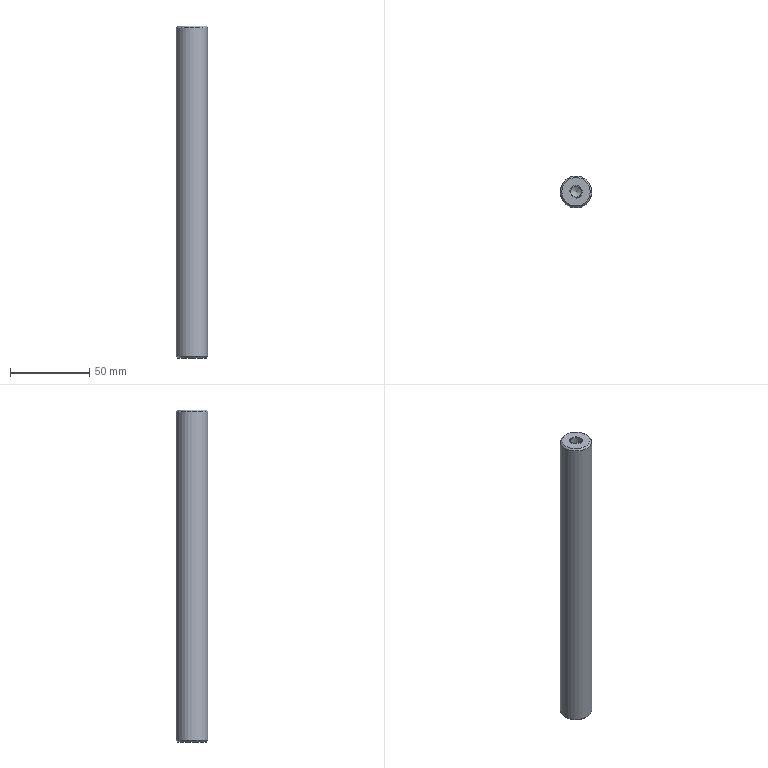Part | STEP file | DP20X210 | 1 solid | 15 faces | box 20 x 20 x 210 mm | volume 65178 mm3 | plane 6 | cone 5 | cylinder 4 | commonest cylinder face diameters 6.8 x1 7.973 x1 8 x1 20 x1
STEP:
#1=CARTESIAN_POINT('',(0.,0.,0.));
#2=DIRECTION('',(0.,0.,1.));
#3=DIRECTION('',(1.,0.,0.));
#4=AXIS2_PLACEMENT_3D('',#1,#2,#3);
#5=CARTESIAN_POINT('',(141.,-270.,341.));
#6=VERTEX_POINT('',#5);
#7=CARTESIAN_POINT('',(132.,-270.,341.));
#8=DIRECTION('',(0.,0.,1.));
#9=DIRECTION('',(1.,0.,0.));
#10=AXIS2_PLACEMENT_3D('',#7,#8,#9);
#11=CIRCLE('',#10,9.);
#12=CARTESIAN_POINT('',(132.,-270.,341.));
#13=DIRECTION('',(0.,0.,1.));
#14=DIRECTION('',(1.,0.,0.));
#15=AXIS2_PLACEMENT_3D('',#12,#13,#14);
#16=PLANE('',#15);
#17=CARTESIAN_POINT('',(0.,0.));
#18=DIRECTION('',(1.,0.));
#19=AXIS2_PLACEMENT_2D('',#17,#18);
#20=CIRCLE('',#19,9.);
#21=(GEOMETRIC_REPRESENTATION_CONTEXT(2)PARAMETRIC_REPRESENTATION_CONTEXT()REPRESENTATION_CONTEXT('',''));
#22=DEFINITIONAL_REPRESENTATION('',(#20),#21);
#23=PCURVE('',#16,#22);
#24=CARTESIAN_POINT('',(132.,-270.,340.));
#25=DIRECTION('',(0.,0.,-1.));
#26=DIRECTION('',(-1.,0.,0.));
#27=AXIS2_PLACEMENT_3D('',#24,#25,#26);
#28=CONICAL_SURFACE('',#27,10.,0.7854);
#29=CARTESIAN_POINT('',(9.425,-1.));
#30=DIRECTION('',(-1.,0.));
#31=VECTOR('',#30,1.);
#32=LINE('',#29,#31);
#33=(GEOMETRIC_REPRESENTATION_CONTEXT(2)PARAMETRIC_REPRESENTATION_CONTEXT()REPRESENTATION_CONTEXT('',''));
#34=DEFINITIONAL_REPRESENTATION('',(#32),#33);
#35=PCURVE('',#28,#34);
#36=SURFACE_CURVE('',#11,(#23,#35),.PCURVE_S1.);
#37=EDGE_CURVE('',#6,#6,#36,.T.);
#38=ORIENTED_EDGE('',*,*,#37,.T.);
#39=EDGE_LOOP('',(#38));
#40=FACE_BOUND('',#39,.T.);
#41=CARTESIAN_POINT('',(128.,-270.,341.));
#42=VERTEX_POINT('',#41);
#43=CARTESIAN_POINT('',(128.013,-270.,341.));
#44=VERTEX_POINT('',#43);
#45=CARTESIAN_POINT('',(132.,-270.,341.));
#46=DIRECTION('',(1.,0.,0.));
#47=VECTOR('',#46,1.);
#48=LINE('',#45,#47);
#49=CARTESIAN_POINT('',(0.,0.));
#50=DIRECTION('',(1.,0.));
#51=VECTOR('',#50,1.);
#52=LINE('',#49,#51);
#53=(GEOMETRIC_REPRESENTATION_CONTEXT(2)PARAMETRIC_REPRESENTATION_CONTEXT()REPRESENTATION_CONTEXT('',''));
#54=DEFINITIONAL_REPRESENTATION('',(#52),#53);
#55=PCURVE('',#16,#54);
#56=CARTESIAN_POINT('',(132.,-270.,365.333));
#57=DIRECTION('',(0.,1.,0.));
#58=DIRECTION('',(0.,0.,1.));
#59=AXIS2_PLACEMENT_3D('',#56,#57,#58);
#60=PLANE('',#59);
#61=CARTESIAN_POINT('',(-24.333,0.));
#62=DIRECTION('',(0.,1.));
#63=VECTOR('',#62,1.);
#64=LINE('',#61,#63);
#65=(GEOMETRIC_REPRESENTATION_CONTEXT(2)PARAMETRIC_REPRESENTATION_CONTEXT()REPRESENTATION_CONTEXT('',''));
#66=DEFINITIONAL_REPRESENTATION('',(#64),#65);
#67=PCURVE('',#60,#66);
#68=SURFACE_CURVE('',#48,(#55,#67),.PCURVE_S1.);
#69=EDGE_CURVE('',#42,#44,#68,.T.);
#70=ORIENTED_EDGE('',*,*,#69,.F.);
#71=CARTESIAN_POINT('',(132.,-274.,341.));
#72=VERTEX_POINT('',#71);
#73=CARTESIAN_POINT('',(132.,-270.,341.));
#74=DIRECTION('',(0.,0.,1.));
#75=DIRECTION('',(0.,1.,0.));
#76=AXIS2_PLACEMENT_3D('',#73,#74,#75);
#77=CIRCLE('',#76,4.);
#78=CARTESIAN_POINT('',(0.,0.));
#79=DIRECTION('',(0.,1.));
#80=AXIS2_PLACEMENT_2D('',#78,#79);
#81=CIRCLE('',#80,4.);
#82=(GEOMETRIC_REPRESENTATION_CONTEXT(2)PARAMETRIC_REPRESENTATION_CONTEXT()REPRESENTATION_CONTEXT('',''));
#83=DEFINITIONAL_REPRESENTATION('',(#81),#82);
#84=PCURVE('',#16,#83);
#85=CARTESIAN_POINT('',(132.,-270.,323.667));
#86=DIRECTION('',(0.,0.,1.));
#87=DIRECTION('',(1.,0.,0.));
#88=AXIS2_PLACEMENT_3D('',#85,#86,#87);
#89=CYLINDRICAL_SURFACE('',#88,4.);
#90=CARTESIAN_POINT('',(-4.712,17.333));
#91=DIRECTION('',(1.,0.));
#92=VECTOR('',#91,1.);
#93=LINE('',#90,#92);
#94=(GEOMETRIC_REPRESENTATION_CONTEXT(2)PARAMETRIC_REPRESENTATION_CONTEXT()REPRESENTATION_CONTEXT('',''));
#95=DEFINITIONAL_REPRESENTATION('',(#93),#94);
#96=PCURVE('',#89,#95);
#97=SURFACE_CURVE('',#77,(#84,#96),.PCURVE_S1.);
#98=EDGE_CURVE('',#72,#42,#97,.T.);
#99=ORIENTED_EDGE('',*,*,#98,.F.);
#100=CARTESIAN_POINT('',(132.,-273.987,341.));
#101=VERTEX_POINT('',#100);
#102=CARTESIAN_POINT('',(132.,-270.,341.));
#103=DIRECTION('',(0.,-1.,0.));
#104=VECTOR('',#103,1.);
#105=LINE('',#102,#104);
#106=CARTESIAN_POINT('',(0.,0.));
#107=DIRECTION('',(0.,-1.));
#108=VECTOR('',#107,1.);
#109=LINE('',#106,#108);
#110=(GEOMETRIC_REPRESENTATION_CONTEXT(2)PARAMETRIC_REPRESENTATION_CONTEXT()REPRESENTATION_CONTEXT('',''));
#111=DEFINITIONAL_REPRESENTATION('',(#109),#110);
#112=PCURVE('',#16,#111);
#113=CARTESIAN_POINT('',(132.,-270.,362.333));
#114=DIRECTION('',(1.,0.,0.));
#115=DIRECTION('',(0.,0.,-1.));
#116=AXIS2_PLACEMENT_3D('',#113,#114,#115);
#117=PLANE('',#116);
#118=CARTESIAN_POINT('',(21.333,0.));
#119=DIRECTION('',(0.,-1.));
#120=VECTOR('',#119,1.);
#121=LINE('',#118,#120);
#122=(GEOMETRIC_REPRESENTATION_CONTEXT(2)PARAMETRIC_REPRESENTATION_CONTEXT()REPRESENTATION_CONTEXT('',''));
#123=DEFINITIONAL_REPRESENTATION('',(#121),#122);
#124=PCURVE('',#117,#123);
#125=SURFACE_CURVE('',#105,(#112,#124),.PCURVE_S1.);
#126=EDGE_CURVE('',#101,#72,#125,.T.);
#127=ORIENTED_EDGE('',*,*,#126,.F.);
#128=CARTESIAN_POINT('',(132.,-270.,341.));
#129=DIRECTION('',(0.,0.,1.));
#130=DIRECTION('',(1.,0.,0.));
#131=AXIS2_PLACEMENT_3D('',#128,#129,#130);
#132=CIRCLE('',#131,3.987);
#133=CARTESIAN_POINT('',(0.,0.));
#134=DIRECTION('',(1.,0.));
#135=AXIS2_PLACEMENT_2D('',#133,#134);
#136=CIRCLE('',#135,3.987);
#137=(GEOMETRIC_REPRESENTATION_CONTEXT(2)PARAMETRIC_REPRESENTATION_CONTEXT()REPRESENTATION_CONTEXT('',''));
#138=DEFINITIONAL_REPRESENTATION('',(#136),#137);
#139=PCURVE('',#16,#138);
#140=CARTESIAN_POINT('',(132.,-270.,323.667));
#141=DIRECTION('',(0.,0.,1.));
#142=DIRECTION('',(1.,0.,0.));
#143=AXIS2_PLACEMENT_3D('',#140,#141,#142);
#144=CYLINDRICAL_SURFACE('',#143,3.987);
#145=CARTESIAN_POINT('',(-6.283,17.333));
#146=DIRECTION('',(1.,0.));
#147=VECTOR('',#146,1.);
#148=LINE('',#145,#147);
#149=(GEOMETRIC_REPRESENTATION_CONTEXT(2)PARAMETRIC_REPRESENTATION_CONTEXT()REPRESENTATION_CONTEXT('',''));
#150=DEFINITIONAL_REPRESENTATION('',(#148),#149);
#151=PCURVE('',#144,#150);
#152=SURFACE_CURVE('',#132,(#139,#151),.PCURVE_S1.);
#153=EDGE_CURVE('',#101,#44,#152,.T.);
#154=ORIENTED_EDGE('',*,*,#153,.T.);
#155=EDGE_LOOP('',(#70,#99,#127,#154));
#156=FACE_BOUND('',#155,.T.);
#157=CARTESIAN_POINT('',(128.6,-270.,341.));
#158=VERTEX_POINT('',#157);
#159=CARTESIAN_POINT('',(135.4,-270.,341.));
#160=VERTEX_POINT('',#159);
#161=CARTESIAN_POINT('',(132.,-270.,341.));
#162=DIRECTION('',(0.,0.,-1.));
#163=DIRECTION('',(-1.,0.,0.));
#164=AXIS2_PLACEMENT_3D('',#161,#162,#163);
#165=CIRCLE('',#164,3.4);
#166=CARTESIAN_POINT('',(-3.4,0.));
#167=CARTESIAN_POINT('',(-3.4,5.889));
#168=CARTESIAN_POINT('',(1.7,2.944));
#169=CARTESIAN_POINT('',(6.8,0.));
#170=CARTESIAN_POINT('',(1.7,-2.944));
#171=CARTESIAN_POINT('',(-3.4,-5.889));
#172=CARTESIAN_POINT('',(-3.4,0.));
#173=(BOUNDED_CURVE()B_SPLINE_CURVE(2,(#166,#167,#168,#169,#170,#171,#172),.UNSPECIFIED.,.T.,.F.)B_SPLINE_CURVE_WITH_KNOTS((1,2,2,2,2,1),(-2.094,0.,2.094,4.189,6.283,8.378),.UNSPECIFIED.)CURVE()GEOMETRIC_REPRESENTATION_ITEM()RATIONAL_B_SPLINE_CURVE((1.,0.5,1.,0.5,1.,0.5,1.))REPRESENTATION_ITEM(''));
#174=(GEOMETRIC_REPRESENTATION_CONTEXT(2)PARAMETRIC_REPRESENTATION_CONTEXT()REPRESENTATION_CONTEXT('',''));
#175=DEFINITIONAL_REPRESENTATION('',(#173),#174);
#176=PCURVE('',#16,#175);
#177=CARTESIAN_POINT('',(132.,-270.,318.637));
#178=DIRECTION('',(0.,0.,-1.));
#179=DIRECTION('',(0.,1.,0.));
#180=AXIS2_PLACEMENT_3D('',#177,#178,#179);
#181=CYLINDRICAL_SURFACE('',#180,3.4);
#182=CARTESIAN_POINT('',(4.712,-22.363));
#183=DIRECTION('',(1.,0.));
#184=VECTOR('',#183,1.);
#185=LINE('',#182,#184);
#186=(GEOMETRIC_REPRESENTATION_CONTEXT(2)PARAMETRIC_REPRESENTATION_CONTEXT()REPRESENTATION_CONTEXT('',''));
#187=DEFINITIONAL_REPRESENTATION('',(#185),#186);
#188=PCURVE('',#181,#187);
#189=SURFACE_CURVE('',#165,(#176,#188),.PCURVE_S1.);
#190=EDGE_CURVE('',#158,#160,#189,.T.);
#191=ORIENTED_EDGE('',*,*,#190,.T.);
#192=CARTESIAN_POINT('',(132.,-270.,341.));
#193=DIRECTION('',(0.,0.,-1.));
#194=DIRECTION('',(-1.,0.,0.));
#195=AXIS2_PLACEMENT_3D('',#192,#193,#194);
#196=CIRCLE('',#195,3.4);
#197=CARTESIAN_POINT('',(-3.4,0.));
#198=CARTESIAN_POINT('',(-3.4,5.889));
#199=CARTESIAN_POINT('',(1.7,2.944));
#200=CARTESIAN_POINT('',(6.8,0.));
#201=CARTESIAN_POINT('',(1.7,-2.944));
#202=CARTESIAN_POINT('',(-3.4,-5.889));
#203=CARTESIAN_POINT('',(-3.4,0.));
#204=(BOUNDED_CURVE()B_SPLINE_CURVE(2,(#197,#198,#199,#200,#201,#202,#203),.UNSPECIFIED.,.T.,.F.)B_SPLINE_CURVE_WITH_KNOTS((1,2,2,2,2,1),(-2.094,0.,2.094,4.189,6.283,8.378),.UNSPECIFIED.)CURVE()GEOMETRIC_REPRESENTATION_ITEM()RATIONAL_B_SPLINE_CURVE((1.,0.5,1.,0.5,1.,0.5,1.))REPRESENTATION_ITEM(''));
#205=(GEOMETRIC_REPRESENTATION_CONTEXT(2)PARAMETRIC_REPRESENTATION_CONTEXT()REPRESENTATION_CONTEXT('',''));
#206=DEFINITIONAL_REPRESENTATION('',(#204),#205);
#207=PCURVE('',#16,#206);
#208=CARTESIAN_POINT('',(-1.571,-22.363));
#209=DIRECTION('',(1.,0.));
#210=VECTOR('',#209,1.);
#211=LINE('',#208,#210);
#212=(GEOMETRIC_REPRESENTATION_CONTEXT(2)PARAMETRIC_REPRESENTATION_CONTEXT()REPRESENTATION_CONTEXT('',''));
#213=DEFINITIONAL_REPRESENTATION('',(#211),#212);
#214=PCURVE('',#181,#213);
#215=SURFACE_CURVE('',#196,(#207,#214),.PCURVE_S1.);
#216=EDGE_CURVE('',#160,#158,#215,.T.);
#217=ORIENTED_EDGE('',*,*,#216,.T.);
#218=EDGE_LOOP('',(#191,#217));
#219=FACE_BOUND('',#218,.T.);
#220=ADVANCED_FACE('',(#40,#156,#219),#16,.T.);
#221=CARTESIAN_POINT('',(123.,-270.,131.));
#222=VERTEX_POINT('',#221);
#223=CARTESIAN_POINT('',(132.,-270.,131.));
#224=DIRECTION('',(0.,0.,-1.));
#225=DIRECTION('',(-1.,0.,0.));
#226=AXIS2_PLACEMENT_3D('',#223,#224,#225);
#227=CIRCLE('',#226,9.);
#228=CARTESIAN_POINT('',(132.,-270.,131.));
#229=DIRECTION('',(0.,0.,-1.));
#230=DIRECTION('',(-1.,0.,0.));
#231=AXIS2_PLACEMENT_3D('',#228,#229,#230);
#232=PLANE('',#231);
#233=CARTESIAN_POINT('',(0.,0.));
#234=DIRECTION('',(1.,0.));
#235=AXIS2_PLACEMENT_2D('',#233,#234);
#236=CIRCLE('',#235,9.);
#237=(GEOMETRIC_REPRESENTATION_CONTEXT(2)PARAMETRIC_REPRESENTATION_CONTEXT()REPRESENTATION_CONTEXT('',''));
#238=DEFINITIONAL_REPRESENTATION('',(#236),#237);
#239=PCURVE('',#232,#238);
#240=CARTESIAN_POINT('',(132.,-270.,132.));
#241=DIRECTION('',(0.,0.,1.));
#242=DIRECTION('',(1.,0.,0.));
#243=AXIS2_PLACEMENT_3D('',#240,#241,#242);
#244=CONICAL_SURFACE('',#243,10.,0.7854);
#245=CARTESIAN_POINT('',(9.425,-1.));
#246=DIRECTION('',(-1.,0.));
#247=VECTOR('',#246,1.);
#248=LINE('',#245,#247);
#249=(GEOMETRIC_REPRESENTATION_CONTEXT(2)PARAMETRIC_REPRESENTATION_CONTEXT()REPRESENTATION_CONTEXT('',''));
#250=DEFINITIONAL_REPRESENTATION('',(#248),#249);
#251=PCURVE('',#244,#250);
#252=SURFACE_CURVE('',#227,(#239,#251),.PCURVE_S1.);
#253=EDGE_CURVE('',#222,#222,#252,.T.);
#254=ORIENTED_EDGE('',*,*,#253,.T.);
#255=EDGE_LOOP('',(#254));
#256=FACE_BOUND('',#255,.T.);
#257=ADVANCED_FACE('',(#256),#232,.T.);
#258=CARTESIAN_POINT('',(142.,-270.,340.));
#259=VERTEX_POINT('',#258);
#260=CARTESIAN_POINT('',(122.,-270.,340.));
#261=VERTEX_POINT('',#260);
#262=CARTESIAN_POINT('',(132.,-270.,340.));
#263=DIRECTION('',(0.,0.,-1.));
#264=DIRECTION('',(1.,0.,0.));
#265=AXIS2_PLACEMENT_3D('',#262,#263,#264);
#266=CIRCLE('',#265,10.);
#267=CARTESIAN_POINT('',(132.,-270.,341.));
#268=DIRECTION('',(0.,0.,-1.));
#269=DIRECTION('',(-1.,0.,0.));
#270=AXIS2_PLACEMENT_3D('',#267,#268,#269);
#271=CYLINDRICAL_SURFACE('',#270,10.);
#272=CARTESIAN_POINT('',(3.142,1.));
#273=DIRECTION('',(1.,0.));
#274=VECTOR('',#273,1.);
#275=LINE('',#272,#274);
#276=(GEOMETRIC_REPRESENTATION_CONTEXT(2)PARAMETRIC_REPRESENTATION_CONTEXT()REPRESENTATION_CONTEXT('',''));
#277=DEFINITIONAL_REPRESENTATION('',(#275),#276);
#278=PCURVE('',#271,#277);
#279=CARTESIAN_POINT('',(3.142,0.));
#280=DIRECTION('',(1.,0.));
#281=VECTOR('',#280,1.);
#282=LINE('',#279,#281);
#283=(GEOMETRIC_REPRESENTATION_CONTEXT(2)PARAMETRIC_REPRESENTATION_CONTEXT()REPRESENTATION_CONTEXT('',''));
#284=DEFINITIONAL_REPRESENTATION('',(#282),#283);
#285=PCURVE('',#28,#284);
#286=SURFACE_CURVE('',#266,(#278,#285),.PCURVE_S1.);
#287=EDGE_CURVE('',#259,#261,#286,.T.);
#288=ORIENTED_EDGE('',*,*,#287,.T.);
#289=CARTESIAN_POINT('',(122.,-270.,132.));
#290=VERTEX_POINT('',#289);
#291=CARTESIAN_POINT('',(122.,-270.,340.));
#292=CARTESIAN_POINT('',(122.,-270.,132.));
#293=B_SPLINE_CURVE_WITH_KNOTS('',1,(#291,#292),.UNSPECIFIED.,.F.,.F.,(2,2),(1.,209.),.PIECEWISE_BEZIER_KNOTS.);
#294=CARTESIAN_POINT('',(6.283,0.));
#295=DIRECTION('',(0.,1.));
#296=VECTOR('',#295,1.);
#297=LINE('',#294,#296);
#298=(GEOMETRIC_REPRESENTATION_CONTEXT(2)PARAMETRIC_REPRESENTATION_CONTEXT()REPRESENTATION_CONTEXT('',''));
#299=DEFINITIONAL_REPRESENTATION('',(#297),#298);
#300=PCURVE('',#271,#299);
#301=CARTESIAN_POINT('',(0.,0.));
#302=DIRECTION('',(0.,1.));
#303=VECTOR('',#302,1.);
#304=LINE('',#301,#303);
#305=(GEOMETRIC_REPRESENTATION_CONTEXT(2)PARAMETRIC_REPRESENTATION_CONTEXT()REPRESENTATION_CONTEXT('',''));
#306=DEFINITIONAL_REPRESENTATION('',(#304),#305);
#307=PCURVE('',#271,#306);
#308=SEAM_CURVE('',#293,(#300,#307),.PCURVE_S1.);
#309=EDGE_CURVE('',#261,#290,#308,.T.);
#310=ORIENTED_EDGE('',*,*,#309,.T.);
#311=CARTESIAN_POINT('',(132.,-270.,132.));
#312=DIRECTION('',(0.,0.,1.));
#313=DIRECTION('',(-1.,0.,0.));
#314=AXIS2_PLACEMENT_3D('',#311,#312,#313);
#315=CIRCLE('',#314,10.);
#316=CARTESIAN_POINT('',(6.283,209.));
#317=DIRECTION('',(-1.,0.));
#318=VECTOR('',#317,1.);
#319=LINE('',#316,#318);
#320=(GEOMETRIC_REPRESENTATION_CONTEXT(2)PARAMETRIC_REPRESENTATION_CONTEXT()REPRESENTATION_CONTEXT('',''));
#321=DEFINITIONAL_REPRESENTATION('',(#319),#320);
#322=PCURVE('',#271,#321);
#323=CARTESIAN_POINT('',(3.142,0.));
#324=DIRECTION('',(1.,0.));
#325=VECTOR('',#324,1.);
#326=LINE('',#323,#325);
#327=(GEOMETRIC_REPRESENTATION_CONTEXT(2)PARAMETRIC_REPRESENTATION_CONTEXT()REPRESENTATION_CONTEXT('',''));
#328=DEFINITIONAL_REPRESENTATION('',(#326),#327);
#329=PCURVE('',#244,#328);
#330=SURFACE_CURVE('',#315,(#322,#329),.PCURVE_S1.);
#331=EDGE_CURVE('',#290,#290,#330,.T.);
#332=ORIENTED_EDGE('',*,*,#331,.T.);
#333=ORIENTED_EDGE('',*,*,#309,.F.);
#334=CARTESIAN_POINT('',(132.,-270.,340.));
#335=DIRECTION('',(0.,0.,-1.));
#336=DIRECTION('',(1.,0.,0.));
#337=AXIS2_PLACEMENT_3D('',#334,#335,#336);
#338=CIRCLE('',#337,10.);
#339=CARTESIAN_POINT('',(-3.142,1.));
#340=DIRECTION('',(1.,0.));
#341=VECTOR('',#340,1.);
#342=LINE('',#339,#341);
#343=(GEOMETRIC_REPRESENTATION_CONTEXT(2)PARAMETRIC_REPRESENTATION_CONTEXT()REPRESENTATION_CONTEXT('',''));
#344=DEFINITIONAL_REPRESENTATION('',(#342),#343);
#345=PCURVE('',#271,#344);
#346=CARTESIAN_POINT('',(3.142,0.));
#347=DIRECTION('',(1.,0.));
#348=VECTOR('',#347,1.);
#349=LINE('',#346,#348);
#350=(GEOMETRIC_REPRESENTATION_CONTEXT(2)PARAMETRIC_REPRESENTATION_CONTEXT()REPRESENTATION_CONTEXT('',''));
#351=DEFINITIONAL_REPRESENTATION('',(#349),#350);
#352=PCURVE('',#28,#351);
#353=SURFACE_CURVE('',#338,(#345,#352),.PCURVE_S1.);
#354=EDGE_CURVE('',#261,#259,#353,.T.);
#355=ORIENTED_EDGE('',*,*,#354,.T.);
#356=EDGE_LOOP('',(#288,#310,#332,#333,#355));
#357=FACE_BOUND('',#356,.T.);
#358=ADVANCED_FACE('',(#357),#271,.T.);
#359=ORIENTED_EDGE('',*,*,#37,.F.);
#360=CARTESIAN_POINT('',(141.,-270.,341.));
#361=CARTESIAN_POINT('',(142.,-270.,340.));
#362=B_SPLINE_CURVE_WITH_KNOTS('',1,(#360,#361),.UNSPECIFIED.,.F.,.F.,(2,2),(-1.414,0.),.PIECEWISE_BEZIER_KNOTS.);
#363=CARTESIAN_POINT('',(9.425,0.));
#364=DIRECTION('',(0.,1.));
#365=VECTOR('',#364,1.);
#366=LINE('',#363,#365);
#367=(GEOMETRIC_REPRESENTATION_CONTEXT(2)PARAMETRIC_REPRESENTATION_CONTEXT()REPRESENTATION_CONTEXT('',''));
#368=DEFINITIONAL_REPRESENTATION('',(#366),#367);
#369=PCURVE('',#28,#368);
#370=CARTESIAN_POINT('',(3.142,0.));
#371=DIRECTION('',(0.,1.));
#372=VECTOR('',#371,1.);
#373=LINE('',#370,#372);
#374=(GEOMETRIC_REPRESENTATION_CONTEXT(2)PARAMETRIC_REPRESENTATION_CONTEXT()REPRESENTATION_CONTEXT('',''));
#375=DEFINITIONAL_REPRESENTATION('',(#373),#374);
#376=PCURVE('',#28,#375);
#377=SEAM_CURVE('',#362,(#369,#376),.PCURVE_S1.);
#378=EDGE_CURVE('',#6,#259,#377,.T.);
#379=ORIENTED_EDGE('',*,*,#378,.T.);
#380=ORIENTED_EDGE('',*,*,#354,.F.);
#381=ORIENTED_EDGE('',*,*,#287,.F.);
#382=ORIENTED_EDGE('',*,*,#378,.F.);
#383=EDGE_LOOP('',(#359,#379,#380,#381,#382));
#384=FACE_BOUND('',#383,.T.);
#385=ADVANCED_FACE('',(#384),#28,.T.);
#386=ORIENTED_EDGE('',*,*,#253,.F.);
#387=CARTESIAN_POINT('',(123.,-270.,131.));
#388=CARTESIAN_POINT('',(122.,-270.,132.));
#389=B_SPLINE_CURVE_WITH_KNOTS('',1,(#387,#388),.UNSPECIFIED.,.F.,.F.,(2,2),(-1.414,0.),.PIECEWISE_BEZIER_KNOTS.);
#390=CARTESIAN_POINT('',(9.425,0.));
#391=DIRECTION('',(0.,1.));
#392=VECTOR('',#391,1.);
#393=LINE('',#390,#392);
#394=(GEOMETRIC_REPRESENTATION_CONTEXT(2)PARAMETRIC_REPRESENTATION_CONTEXT()REPRESENTATION_CONTEXT('',''));
#395=DEFINITIONAL_REPRESENTATION('',(#393),#394);
#396=PCURVE('',#244,#395);
#397=CARTESIAN_POINT('',(3.142,0.));
#398=DIRECTION('',(0.,1.));
#399=VECTOR('',#398,1.);
#400=LINE('',#397,#399);
#401=(GEOMETRIC_REPRESENTATION_CONTEXT(2)PARAMETRIC_REPRESENTATION_CONTEXT()REPRESENTATION_CONTEXT('',''));
#402=DEFINITIONAL_REPRESENTATION('',(#400),#401);
#403=PCURVE('',#244,#402);
#404=SEAM_CURVE('',#389,(#396,#403),.PCURVE_S1.);
#405=EDGE_CURVE('',#222,#290,#404,.T.);
#406=ORIENTED_EDGE('',*,*,#405,.T.);
#407=ORIENTED_EDGE('',*,*,#331,.F.);
#408=ORIENTED_EDGE('',*,*,#405,.F.);
#409=EDGE_LOOP('',(#386,#406,#407,#408));
#410=FACE_BOUND('',#409,.T.);
#411=ADVANCED_FACE('',(#410),#244,.T.);
#412=CARTESIAN_POINT('',(128.007,-270.,324.578));
#413=VERTEX_POINT('',#412);
#414=CARTESIAN_POINT('',(128.6,-270.,323.985));
#415=VERTEX_POINT('',#414);
#416=CARTESIAN_POINT('',(132.,-270.,320.594));
#417=DIRECTION('',(0.7071,0.,-0.7071));
#418=VECTOR('',#417,1.);
#419=LINE('',#416,#418);
#420=CARTESIAN_POINT('',(132.,-270.,361.333));
#421=DIRECTION('',(0.,1.,0.));
#422=DIRECTION('',(0.,0.,1.));
#423=AXIS2_PLACEMENT_3D('',#420,#421,#422);
#424=PLANE('',#423);
#425=CARTESIAN_POINT('',(-40.739,0.));
#426=DIRECTION('',(-0.7071,0.7071));
#427=VECTOR('',#426,1.);
#428=LINE('',#425,#427);
#429=(GEOMETRIC_REPRESENTATION_CONTEXT(2)PARAMETRIC_REPRESENTATION_CONTEXT()REPRESENTATION_CONTEXT('',''));
#430=DEFINITIONAL_REPRESENTATION('',(#428),#429);
#431=PCURVE('',#424,#430);
#432=CARTESIAN_POINT('',(132.,-270.,323.918));
#433=DIRECTION('',(0.,0.,1.));
#434=DIRECTION('',(0.,-1.,0.));
#435=AXIS2_PLACEMENT_3D('',#432,#433,#434);
#436=CONICAL_SURFACE('',#435,3.324,0.7854);
#437=CARTESIAN_POINT('',(4.712,-3.324));
#438=DIRECTION('',(0.,-1.));
#439=VECTOR('',#438,1.);
#440=LINE('',#437,#439);
#441=(GEOMETRIC_REPRESENTATION_CONTEXT(2)PARAMETRIC_REPRESENTATION_CONTEXT()REPRESENTATION_CONTEXT('',''));
#442=DEFINITIONAL_REPRESENTATION('',(#440),#441);
#443=PCURVE('',#436,#442);
#444=SURFACE_CURVE('',#419,(#431,#443),.PCURVE_S1.);
#445=EDGE_CURVE('',#413,#415,#444,.T.);
#446=ORIENTED_EDGE('',*,*,#445,.T.);
#447=CARTESIAN_POINT('',(132.,-270.,320.576));
#448=DIRECTION('',(-0.7071,0.,0.7071));
#449=VECTOR('',#448,1.);
#450=LINE('',#447,#449);
#451=CARTESIAN_POINT('',(-40.758,0.));
#452=DIRECTION('',(0.7071,-0.7071));
#453=VECTOR('',#452,1.);
#454=LINE('',#451,#453);
#455=(GEOMETRIC_REPRESENTATION_CONTEXT(2)PARAMETRIC_REPRESENTATION_CONTEXT()REPRESENTATION_CONTEXT('',''));
#456=DEFINITIONAL_REPRESENTATION('',(#454),#455);
#457=PCURVE('',#424,#456);
#458=CARTESIAN_POINT('',(132.,-270.,323.909));
#459=DIRECTION('',(0.,0.,1.));
#460=DIRECTION('',(0.,-1.,0.));
#461=AXIS2_PLACEMENT_3D('',#458,#459,#460);
#462=CONICAL_SURFACE('',#461,3.333,0.7854);
#463=CARTESIAN_POINT('',(4.712,-3.333));
#464=DIRECTION('',(0.,1.));
#465=VECTOR('',#464,1.);
#466=LINE('',#463,#465);
#467=(GEOMETRIC_REPRESENTATION_CONTEXT(2)PARAMETRIC_REPRESENTATION_CONTEXT()REPRESENTATION_CONTEXT('',''));
#468=DEFINITIONAL_REPRESENTATION('',(#466),#467);
#469=PCURVE('',#462,#468);
#470=SURFACE_CURVE('',#450,(#457,#469),.PCURVE_S1.);
#471=EDGE_CURVE('',#415,#413,#470,.T.);
#472=ORIENTED_EDGE('',*,*,#471,.T.);
#473=EDGE_LOOP('',(#446,#472));
#474=FACE_BOUND('',#473,.T.);
#475=ADVANCED_FACE('',(#474),#424,.T.);
#476=CARTESIAN_POINT('',(132.,-273.993,324.578));
#477=VERTEX_POINT('',#476);
#478=CARTESIAN_POINT('',(132.,-273.4,323.985));
#479=VERTEX_POINT('',#478);
#480=CARTESIAN_POINT('',(132.,-270.,320.576));
#481=DIRECTION('',(0.,0.7071,-0.7071));
#482=VECTOR('',#481,1.);
#483=LINE('',#480,#482);
#484=CARTESIAN_POINT('',(132.,-270.,361.333));
#485=DIRECTION('',(1.,0.,0.));
#486=DIRECTION('',(0.,0.,-1.));
#487=AXIS2_PLACEMENT_3D('',#484,#485,#486);
#488=PLANE('',#487);
#489=CARTESIAN_POINT('',(40.758,0.));
#490=DIRECTION('',(0.7071,0.7071));
#491=VECTOR('',#490,1.);
#492=LINE('',#489,#491);
#493=(GEOMETRIC_REPRESENTATION_CONTEXT(2)PARAMETRIC_REPRESENTATION_CONTEXT()REPRESENTATION_CONTEXT('',''));
#494=DEFINITIONAL_REPRESENTATION('',(#492),#493);
#495=PCURVE('',#488,#494);
#496=CARTESIAN_POINT('',(0.,-3.333));
#497=DIRECTION('',(0.,-1.));
#498=VECTOR('',#497,1.);
#499=LINE('',#496,#498);
#500=(GEOMETRIC_REPRESENTATION_CONTEXT(2)PARAMETRIC_REPRESENTATION_CONTEXT()REPRESENTATION_CONTEXT('',''));
#501=DEFINITIONAL_REPRESENTATION('',(#499),#500);
#502=PCURVE('',#462,#501);
#503=SURFACE_CURVE('',#483,(#495,#502),.PCURVE_S1.);
#504=EDGE_CURVE('',#477,#479,#503,.T.);
#505=ORIENTED_EDGE('',*,*,#504,.T.);
#506=CARTESIAN_POINT('',(132.,-270.,320.594));
#507=DIRECTION('',(0.,-0.7071,0.7071));
#508=VECTOR('',#507,1.);
#509=LINE('',#506,#508);
#510=CARTESIAN_POINT('',(40.739,0.));
#511=DIRECTION('',(-0.7071,-0.7071));
#512=VECTOR('',#511,1.);
#513=LINE('',#510,#512);
#514=(GEOMETRIC_REPRESENTATION_CONTEXT(2)PARAMETRIC_REPRESENTATION_CONTEXT()REPRESENTATION_CONTEXT('',''));
#515=DEFINITIONAL_REPRESENTATION('',(#513),#514);
#516=PCURVE('',#488,#515);
#517=CARTESIAN_POINT('',(0.,-3.324));
#518=DIRECTION('',(0.,1.));
#519=VECTOR('',#518,1.);
#520=LINE('',#517,#519);
#521=(GEOMETRIC_REPRESENTATION_CONTEXT(2)PARAMETRIC_REPRESENTATION_CONTEXT()REPRESENTATION_CONTEXT('',''));
#522=DEFINITIONAL_REPRESENTATION('',(#520),#521);
#523=PCURVE('',#436,#522);
#524=SURFACE_CURVE('',#509,(#516,#523),.PCURVE_S1.);
#525=EDGE_CURVE('',#479,#477,#524,.T.);
#526=ORIENTED_EDGE('',*,*,#525,.T.);
#527=EDGE_LOOP('',(#505,#526));
#528=FACE_BOUND('',#527,.T.);
#529=ADVANCED_FACE('',(#528),#488,.T.);
#530=CARTESIAN_POINT('',(135.4,-270.,321.547));
#531=VERTEX_POINT('',#530);
#532=CARTESIAN_POINT('',(132.,-273.4,321.547));
#533=VERTEX_POINT('',#532);
#534=CARTESIAN_POINT('',(132.,-270.,321.547));
#535=DIRECTION('',(0.,0.,-1.));
#536=DIRECTION('',(1.,0.,0.));
#537=AXIS2_PLACEMENT_3D('',#534,#535,#536);
#538=CIRCLE('',#537,3.4);
#539=CARTESIAN_POINT('',(1.571,-2.91));
#540=DIRECTION('',(1.,0.));
#541=VECTOR('',#540,1.);
#542=LINE('',#539,#541);
#543=(GEOMETRIC_REPRESENTATION_CONTEXT(2)PARAMETRIC_REPRESENTATION_CONTEXT()REPRESENTATION_CONTEXT('',''));
#544=DEFINITIONAL_REPRESENTATION('',(#542),#543);
#545=PCURVE('',#181,#544);
#546=CARTESIAN_POINT('',(132.,-270.,319.584));
#547=DIRECTION('',(0.,0.,1.));
#548=DIRECTION('',(0.,-1.,0.));
#549=AXIS2_PLACEMENT_3D('',#546,#547,#548);
#550=CONICAL_SURFACE('',#549,0.,1.047);
#551=CARTESIAN_POINT('',(1.571,1.963));
#552=DIRECTION('',(-1.,0.));
#553=VECTOR('',#552,1.);
#554=LINE('',#551,#553);
#555=(GEOMETRIC_REPRESENTATION_CONTEXT(2)PARAMETRIC_REPRESENTATION_CONTEXT()REPRESENTATION_CONTEXT('',''));
#556=DEFINITIONAL_REPRESENTATION('',(#554),#555);
#557=PCURVE('',#550,#556);
#558=SURFACE_CURVE('',#538,(#545,#557),.PCURVE_S1.);
#559=EDGE_CURVE('',#531,#533,#558,.T.);
#560=ORIENTED_EDGE('',*,*,#559,.F.);
#561=CARTESIAN_POINT('',(135.4,-270.,323.976));
#562=VERTEX_POINT('',#561);
#563=CARTESIAN_POINT('',(135.4,-270.,323.976));
#564=CARTESIAN_POINT('',(135.4,-270.,321.547));
#565=B_SPLINE_CURVE_WITH_KNOTS('',1,(#563,#564),.UNSPECIFIED.,.F.,.F.,(2,2),(-5.339,-2.91),.PIECEWISE_BEZIER_KNOTS.);
#566=CARTESIAN_POINT('',(1.571,0.));
#567=DIRECTION('',(0.,1.));
#568=VECTOR('',#567,1.);
#569=LINE('',#566,#568);
#570=(GEOMETRIC_REPRESENTATION_CONTEXT(2)PARAMETRIC_REPRESENTATION_CONTEXT()REPRESENTATION_CONTEXT('',''));
#571=DEFINITIONAL_REPRESENTATION('',(#569),#570);
#572=PCURVE('',#181,#571);
#573=CARTESIAN_POINT('',(7.854,0.));
#574=DIRECTION('',(0.,1.));
#575=VECTOR('',#574,1.);
#576=LINE('',#573,#575);
#577=(GEOMETRIC_REPRESENTATION_CONTEXT(2)PARAMETRIC_REPRESENTATION_CONTEXT()REPRESENTATION_CONTEXT('',''));
#578=DEFINITIONAL_REPRESENTATION('',(#576),#577);
#579=PCURVE('',#181,#578);
#580=SEAM_CURVE('',#565,(#572,#579),.PCURVE_S1.);
#581=EDGE_CURVE('',#562,#531,#580,.T.);
#582=ORIENTED_EDGE('',*,*,#581,.F.);
#583=CARTESIAN_POINT('',(132.,-270.,323.976));
#584=DIRECTION('',(0.,0.,-1.));
#585=DIRECTION('',(1.,0.,0.));
#586=AXIS2_PLACEMENT_3D('',#583,#584,#585);
#587=CIRCLE('',#586,3.4);
#588=CARTESIAN_POINT('',(-4.712,-5.339));
#589=DIRECTION('',(1.,0.));
#590=VECTOR('',#589,1.);
#591=LINE('',#588,#590);
#592=(GEOMETRIC_REPRESENTATION_CONTEXT(2)PARAMETRIC_REPRESENTATION_CONTEXT()REPRESENTATION_CONTEXT('',''));
#593=DEFINITIONAL_REPRESENTATION('',(#591),#592);
#594=PCURVE('',#181,#593);
#595=CARTESIAN_POINT('',(7.854,0.06667));
#596=DIRECTION('',(-1.,0.));
#597=VECTOR('',#596,1.);
#598=LINE('',#595,#597);
#599=(GEOMETRIC_REPRESENTATION_CONTEXT(2)PARAMETRIC_REPRESENTATION_CONTEXT()REPRESENTATION_CONTEXT('',''));
#600=DEFINITIONAL_REPRESENTATION('',(#598),#599);
#601=PCURVE('',#462,#600);
#602=SURFACE_CURVE('',#587,(#594,#601),.PCURVE_S1.);
#603=EDGE_CURVE('',#562,#479,#602,.T.);
#604=ORIENTED_EDGE('',*,*,#603,.T.);
#605=CARTESIAN_POINT('',(135.4,-270.,323.994));
#606=VERTEX_POINT('',#605);
#607=CARTESIAN_POINT('',(132.,-270.,323.994));
#608=DIRECTION('',(0.,0.,1.));
#609=DIRECTION('',(1.,0.,0.));
#610=AXIS2_PLACEMENT_3D('',#607,#608,#609);
#611=CIRCLE('',#610,3.4);
#612=CARTESIAN_POINT('',(7.854,-5.357));
#613=DIRECTION('',(-1.,0.));
#614=VECTOR('',#613,1.);
#615=LINE('',#612,#614);
#616=(GEOMETRIC_REPRESENTATION_CONTEXT(2)PARAMETRIC_REPRESENTATION_CONTEXT()REPRESENTATION_CONTEXT('',''));
#617=DEFINITIONAL_REPRESENTATION('',(#615),#616);
#618=PCURVE('',#181,#617);
#619=CARTESIAN_POINT('',(-4.712,0.07609));
#620=DIRECTION('',(1.,0.));
#621=VECTOR('',#620,1.);
#622=LINE('',#619,#621);
#623=(GEOMETRIC_REPRESENTATION_CONTEXT(2)PARAMETRIC_REPRESENTATION_CONTEXT()REPRESENTATION_CONTEXT('',''));
#624=DEFINITIONAL_REPRESENTATION('',(#622),#623);
#625=PCURVE('',#436,#624);
#626=SURFACE_CURVE('',#611,(#618,#625),.PCURVE_S1.);
#627=EDGE_CURVE('',#479,#606,#626,.T.);
#628=ORIENTED_EDGE('',*,*,#627,.T.);
#629=CARTESIAN_POINT('',(135.4,-270.,341.));
#630=CARTESIAN_POINT('',(135.4,-270.,323.994));
#631=B_SPLINE_CURVE_WITH_KNOTS('',1,(#629,#630),.UNSPECIFIED.,.F.,.F.,(2,2),(-22.363,-5.357),.PIECEWISE_BEZIER_KNOTS.);
#632=CARTESIAN_POINT('',(1.571,0.));
#633=DIRECTION('',(0.,1.));
#634=VECTOR('',#633,1.);
#635=LINE('',#632,#634);
#636=(GEOMETRIC_REPRESENTATION_CONTEXT(2)PARAMETRIC_REPRESENTATION_CONTEXT()REPRESENTATION_CONTEXT('',''));
#637=DEFINITIONAL_REPRESENTATION('',(#635),#636);
#638=PCURVE('',#181,#637);
#639=CARTESIAN_POINT('',(7.854,0.));
#640=DIRECTION('',(0.,1.));
#641=VECTOR('',#640,1.);
#642=LINE('',#639,#641);
#643=(GEOMETRIC_REPRESENTATION_CONTEXT(2)PARAMETRIC_REPRESENTATION_CONTEXT()REPRESENTATION_CONTEXT('',''));
#644=DEFINITIONAL_REPRESENTATION('',(#642),#643);
#645=PCURVE('',#181,#644);
#646=SEAM_CURVE('',#631,(#638,#645),.PCURVE_S1.);
#647=EDGE_CURVE('',#160,#606,#646,.T.);
#648=ORIENTED_EDGE('',*,*,#647,.F.);
#649=ORIENTED_EDGE('',*,*,#216,.T.);
#650=ORIENTED_EDGE('',*,*,#190,.T.);
#651=ORIENTED_EDGE('',*,*,#647,.T.);
#652=CARTESIAN_POINT('',(132.,-270.,323.994));
#653=DIRECTION('',(0.,0.,1.));
#654=DIRECTION('',(1.,0.,0.));
#655=AXIS2_PLACEMENT_3D('',#652,#653,#654);
#656=CIRCLE('',#655,3.4);
#657=CARTESIAN_POINT('',(14.137,-5.357));
#658=DIRECTION('',(-1.,0.));
#659=VECTOR('',#658,1.);
#660=LINE('',#657,#659);
#661=(GEOMETRIC_REPRESENTATION_CONTEXT(2)PARAMETRIC_REPRESENTATION_CONTEXT()REPRESENTATION_CONTEXT('',''));
#662=DEFINITIONAL_REPRESENTATION('',(#660),#661);
#663=PCURVE('',#181,#662);
#664=CARTESIAN_POINT('',(-4.712,0.07609));
#665=DIRECTION('',(1.,0.));
#666=VECTOR('',#665,1.);
#667=LINE('',#664,#666);
#668=(GEOMETRIC_REPRESENTATION_CONTEXT(2)PARAMETRIC_REPRESENTATION_CONTEXT()REPRESENTATION_CONTEXT('',''));
#669=DEFINITIONAL_REPRESENTATION('',(#667),#668);
#670=PCURVE('',#436,#669);
#671=SURFACE_CURVE('',#656,(#663,#670),.PCURVE_S1.);
#672=EDGE_CURVE('',#606,#415,#671,.T.);
#673=ORIENTED_EDGE('',*,*,#672,.T.);
#674=CARTESIAN_POINT('',(132.,-270.,323.976));
#675=DIRECTION('',(0.,0.,-1.));
#676=DIRECTION('',(1.,0.,0.));
#677=AXIS2_PLACEMENT_3D('',#674,#675,#676);
#678=CIRCLE('',#677,3.4);
#679=CARTESIAN_POINT('',(1.571,-5.339));
#680=DIRECTION('',(1.,0.));
#681=VECTOR('',#680,1.);
#682=LINE('',#679,#681);
#683=(GEOMETRIC_REPRESENTATION_CONTEXT(2)PARAMETRIC_REPRESENTATION_CONTEXT()REPRESENTATION_CONTEXT('',''));
#684=DEFINITIONAL_REPRESENTATION('',(#682),#683);
#685=PCURVE('',#181,#684);
#686=CARTESIAN_POINT('',(7.854,0.06667));
#687=DIRECTION('',(-1.,0.));
#688=VECTOR('',#687,1.);
#689=LINE('',#686,#688);
#690=(GEOMETRIC_REPRESENTATION_CONTEXT(2)PARAMETRIC_REPRESENTATION_CONTEXT()REPRESENTATION_CONTEXT('',''));
#691=DEFINITIONAL_REPRESENTATION('',(#689),#690);
#692=PCURVE('',#462,#691);
#693=SURFACE_CURVE('',#678,(#685,#692),.PCURVE_S1.);
#694=EDGE_CURVE('',#415,#562,#693,.T.);
#695=ORIENTED_EDGE('',*,*,#694,.T.);
#696=ORIENTED_EDGE('',*,*,#581,.T.);
#697=CARTESIAN_POINT('',(132.,-270.,321.547));
#698=DIRECTION('',(0.,0.,-1.));
#699=DIRECTION('',(1.,0.,0.));
#700=AXIS2_PLACEMENT_3D('',#697,#698,#699);
#701=CIRCLE('',#700,3.4);
#702=CARTESIAN_POINT('',(1.571,-2.91));
#703=DIRECTION('',(1.,0.));
#704=VECTOR('',#703,1.);
#705=LINE('',#702,#704);
#706=(GEOMETRIC_REPRESENTATION_CONTEXT(2)PARAMETRIC_REPRESENTATION_CONTEXT()REPRESENTATION_CONTEXT('',''));
#707=DEFINITIONAL_REPRESENTATION('',(#705),#706);
#708=PCURVE('',#181,#707);
#709=CARTESIAN_POINT('',(7.854,1.963));
#710=DIRECTION('',(-1.,0.));
#711=VECTOR('',#710,1.);
#712=LINE('',#709,#711);
#713=(GEOMETRIC_REPRESENTATION_CONTEXT(2)PARAMETRIC_REPRESENTATION_CONTEXT()REPRESENTATION_CONTEXT('',''));
#714=DEFINITIONAL_REPRESENTATION('',(#712),#713);
#715=PCURVE('',#550,#714);
#716=SURFACE_CURVE('',#701,(#708,#715),.PCURVE_S1.);
#717=EDGE_CURVE('',#533,#531,#716,.T.);
#718=ORIENTED_EDGE('',*,*,#717,.F.);
#719=EDGE_LOOP('',(#560,#582,#604,#628,#648,#649,#650,#651,#673,#695,#696,#718));
#720=FACE_BOUND('',#719,.F.);
#721=ADVANCED_FACE('',(#720),#181,.F.);
#722=CARTESIAN_POINT('',(132.,-270.,324.581));
#723=DIRECTION('',(0.,0.,-1.));
#724=DIRECTION('',(1.,0.,0.));
#725=AXIS2_PLACEMENT_3D('',#722,#723,#724);
#726=CIRCLE('',#725,3.987);
#727=CARTESIAN_POINT('',(6.283,0.9145));
#728=DIRECTION('',(-1.,0.));
#729=VECTOR('',#728,1.);
#730=LINE('',#727,#729);
#731=(GEOMETRIC_REPRESENTATION_CONTEXT(2)PARAMETRIC_REPRESENTATION_CONTEXT()REPRESENTATION_CONTEXT('',''));
#732=DEFINITIONAL_REPRESENTATION('',(#730),#731);
#733=PCURVE('',#144,#732);
#734=CARTESIAN_POINT('',(7.854,0.6628));
#735=DIRECTION('',(-1.,0.));
#736=VECTOR('',#735,1.);
#737=LINE('',#734,#736);
#738=(GEOMETRIC_REPRESENTATION_CONTEXT(2)PARAMETRIC_REPRESENTATION_CONTEXT()REPRESENTATION_CONTEXT('',''));
#739=DEFINITIONAL_REPRESENTATION('',(#737),#738);
#740=PCURVE('',#436,#739);
#741=SURFACE_CURVE('',#726,(#733,#740),.PCURVE_S1.);
#742=EDGE_CURVE('',#413,#477,#741,.T.);
#743=ORIENTED_EDGE('',*,*,#742,.F.);
#744=CARTESIAN_POINT('',(128.013,-270.,326.667));
#745=DIRECTION('',(0.,0.,-1.));
#746=VECTOR('',#745,1.);
#747=LINE('',#744,#746);
#748=CARTESIAN_POINT('',(3.142,3.));
#749=DIRECTION('',(0.,-1.));
#750=VECTOR('',#749,1.);
#751=LINE('',#748,#750);
#752=(GEOMETRIC_REPRESENTATION_CONTEXT(2)PARAMETRIC_REPRESENTATION_CONTEXT()REPRESENTATION_CONTEXT('',''));
#753=DEFINITIONAL_REPRESENTATION('',(#751),#752);
#754=PCURVE('',#144,#753);
#755=CARTESIAN_POINT('',(-38.667,-3.987));
#756=DIRECTION('',(-1.,0.));
#757=VECTOR('',#756,1.);
#758=LINE('',#755,#757);
#759=(GEOMETRIC_REPRESENTATION_CONTEXT(2)PARAMETRIC_REPRESENTATION_CONTEXT()REPRESENTATION_CONTEXT('',''));
#760=DEFINITIONAL_REPRESENTATION('',(#758),#759);
#761=PCURVE('',#60,#760);
#762=SURFACE_CURVE('',#747,(#754,#761),.PCURVE_S1.);
#763=EDGE_CURVE('',#44,#413,#762,.T.);
#764=ORIENTED_EDGE('',*,*,#763,.F.);
#765=ORIENTED_EDGE('',*,*,#153,.F.);
#766=CARTESIAN_POINT('',(132.,-273.987,323.667));
#767=DIRECTION('',(0.,0.,1.));
#768=VECTOR('',#767,1.);
#769=LINE('',#766,#768);
#770=CARTESIAN_POINT('',(-1.571,0.));
#771=DIRECTION('',(0.,1.));
#772=VECTOR('',#771,1.);
#773=LINE('',#770,#772);
#774=(GEOMETRIC_REPRESENTATION_CONTEXT(2)PARAMETRIC_REPRESENTATION_CONTEXT()REPRESENTATION_CONTEXT('',''));
#775=DEFINITIONAL_REPRESENTATION('',(#773),#774);
#776=PCURVE('',#144,#775);
#777=CARTESIAN_POINT('',(38.667,-3.987));
#778=DIRECTION('',(-1.,0.));
#779=VECTOR('',#778,1.);
#780=LINE('',#777,#779);
#781=(GEOMETRIC_REPRESENTATION_CONTEXT(2)PARAMETRIC_REPRESENTATION_CONTEXT()REPRESENTATION_CONTEXT('',''));
#782=DEFINITIONAL_REPRESENTATION('',(#780),#781);
#783=PCURVE('',#117,#782);
#784=SURFACE_CURVE('',#769,(#776,#783),.PCURVE_S1.);
#785=EDGE_CURVE('',#477,#101,#784,.T.);
#786=ORIENTED_EDGE('',*,*,#785,.F.);
#787=EDGE_LOOP('',(#743,#764,#765,#786));
#788=FACE_BOUND('',#787,.T.);
#789=ADVANCED_FACE('',(#788),#144,.T.);
#790=ORIENTED_EDGE('',*,*,#742,.T.);
#791=ORIENTED_EDGE('',*,*,#525,.F.);
#792=ORIENTED_EDGE('',*,*,#627,.T.);
#793=ORIENTED_EDGE('',*,*,#672,.T.);
#794=ORIENTED_EDGE('',*,*,#445,.F.);
#795=EDGE_LOOP('',(#790,#791,#792,#793,#794));
#796=FACE_BOUND('',#795,.T.);
#797=ADVANCED_FACE('',(#796),#436,.T.);
#798=CARTESIAN_POINT('',(132.,-270.,324.576));
#799=DIRECTION('',(0.,0.,1.));
#800=DIRECTION('',(1.,0.,0.));
#801=AXIS2_PLACEMENT_3D('',#798,#799,#800);
#802=CIRCLE('',#801,4.);
#803=CARTESIAN_POINT('',(-4.712,0.6667));
#804=DIRECTION('',(1.,0.));
#805=VECTOR('',#804,1.);
#806=LINE('',#803,#805);
#807=(GEOMETRIC_REPRESENTATION_CONTEXT(2)PARAMETRIC_REPRESENTATION_CONTEXT()REPRESENTATION_CONTEXT('',''));
#808=DEFINITIONAL_REPRESENTATION('',(#806),#807);
#809=PCURVE('',#462,#808);
#810=CARTESIAN_POINT('',(-6.283,0.909));
#811=DIRECTION('',(1.,0.));
#812=VECTOR('',#811,1.);
#813=LINE('',#810,#812);
#814=(GEOMETRIC_REPRESENTATION_CONTEXT(2)PARAMETRIC_REPRESENTATION_CONTEXT()REPRESENTATION_CONTEXT('',''));
#815=DEFINITIONAL_REPRESENTATION('',(#813),#814);
#816=PCURVE('',#89,#815);
#817=SURFACE_CURVE('',#802,(#809,#816),.PCURVE_S1.);
#818=EDGE_CURVE('',#477,#413,#817,.T.);
#819=ORIENTED_EDGE('',*,*,#818,.F.);
#820=ORIENTED_EDGE('',*,*,#504,.T.);
#821=ORIENTED_EDGE('',*,*,#603,.F.);
#822=ORIENTED_EDGE('',*,*,#694,.F.);
#823=ORIENTED_EDGE('',*,*,#471,.T.);
#824=EDGE_LOOP('',(#819,#820,#821,#822,#823));
#825=FACE_BOUND('',#824,.F.);
#826=ADVANCED_FACE('',(#825),#462,.F.);
#827=ORIENTED_EDGE('',*,*,#559,.T.);
#828=CARTESIAN_POINT('',(132.,-270.,319.584));
#829=VERTEX_POINT('',#828);
#830=CARTESIAN_POINT('',(132.,-270.,319.584));
#831=CARTESIAN_POINT('',(132.,-273.4,321.547));
#832=B_SPLINE_CURVE_WITH_KNOTS('',1,(#830,#831),.UNSPECIFIED.,.F.,.F.,(2,2),(0.,3.926),.PIECEWISE_BEZIER_KNOTS.);
#833=CARTESIAN_POINT('',(0.,0.));
#834=DIRECTION('',(0.,1.));
#835=VECTOR('',#834,1.);
#836=LINE('',#833,#835);
#837=(GEOMETRIC_REPRESENTATION_CONTEXT(2)PARAMETRIC_REPRESENTATION_CONTEXT()REPRESENTATION_CONTEXT('',''));
#838=DEFINITIONAL_REPRESENTATION('',(#836),#837);
#839=PCURVE('',#550,#838);
#840=CARTESIAN_POINT('',(6.283,0.));
#841=DIRECTION('',(0.,1.));
#842=VECTOR('',#841,1.);
#843=LINE('',#840,#842);
#844=(GEOMETRIC_REPRESENTATION_CONTEXT(2)PARAMETRIC_REPRESENTATION_CONTEXT()REPRESENTATION_CONTEXT('',''));
#845=DEFINITIONAL_REPRESENTATION('',(#843),#844);
#846=PCURVE('',#550,#845);
#847=SEAM_CURVE('',#832,(#839,#846),.PCURVE_S1.);
#848=EDGE_CURVE('',#829,#533,#847,.T.);
#849=ORIENTED_EDGE('',*,*,#848,.F.);
#850=ORIENTED_EDGE('',*,*,#848,.T.);
#851=ORIENTED_EDGE('',*,*,#717,.T.);
#852=EDGE_LOOP('',(#827,#849,#850,#851));
#853=FACE_BOUND('',#852,.F.);
#854=ADVANCED_FACE('',(#853),#550,.F.);
#855=CARTESIAN_POINT('',(132.,-274.,323.667));
#856=DIRECTION('',(0.,0.,1.));
#857=VECTOR('',#856,1.);
#858=LINE('',#855,#857);
#859=CARTESIAN_POINT('',(-1.571,0.));
#860=DIRECTION('',(0.,1.));
#861=VECTOR('',#860,1.);
#862=LINE('',#859,#861);
#863=(GEOMETRIC_REPRESENTATION_CONTEXT(2)PARAMETRIC_REPRESENTATION_CONTEXT()REPRESENTATION_CONTEXT('',''));
#864=DEFINITIONAL_REPRESENTATION('',(#862),#863);
#865=PCURVE('',#89,#864);
#866=CARTESIAN_POINT('',(38.667,-4.));
#867=DIRECTION('',(-1.,0.));
#868=VECTOR('',#867,1.);
#869=LINE('',#866,#868);
#870=(GEOMETRIC_REPRESENTATION_CONTEXT(2)PARAMETRIC_REPRESENTATION_CONTEXT()REPRESENTATION_CONTEXT('',''));
#871=DEFINITIONAL_REPRESENTATION('',(#869),#870);
#872=PCURVE('',#117,#871);
#873=SURFACE_CURVE('',#858,(#865,#872),.PCURVE_S1.);
#874=EDGE_CURVE('',#477,#72,#873,.T.);
#875=ORIENTED_EDGE('',*,*,#874,.F.);
#876=ORIENTED_EDGE('',*,*,#818,.T.);
#877=CARTESIAN_POINT('',(128.,-270.,326.667));
#878=DIRECTION('',(0.,0.,1.));
#879=VECTOR('',#878,1.);
#880=LINE('',#877,#879);
#881=CARTESIAN_POINT('',(3.142,3.));
#882=DIRECTION('',(0.,1.));
#883=VECTOR('',#882,1.);
#884=LINE('',#881,#883);
#885=(GEOMETRIC_REPRESENTATION_CONTEXT(2)PARAMETRIC_REPRESENTATION_CONTEXT()REPRESENTATION_CONTEXT('',''));
#886=DEFINITIONAL_REPRESENTATION('',(#884),#885);
#887=PCURVE('',#89,#886);
#888=CARTESIAN_POINT('',(-38.667,-4.));
#889=DIRECTION('',(1.,0.));
#890=VECTOR('',#889,1.);
#891=LINE('',#888,#890);
#892=(GEOMETRIC_REPRESENTATION_CONTEXT(2)PARAMETRIC_REPRESENTATION_CONTEXT()REPRESENTATION_CONTEXT('',''));
#893=DEFINITIONAL_REPRESENTATION('',(#891),#892);
#894=PCURVE('',#60,#893);
#895=SURFACE_CURVE('',#880,(#887,#894),.PCURVE_S1.);
#896=EDGE_CURVE('',#413,#42,#895,.T.);
#897=ORIENTED_EDGE('',*,*,#896,.T.);
#898=ORIENTED_EDGE('',*,*,#98,.F.);
#899=EDGE_LOOP('',(#875,#876,#897,#898));
#900=FACE_BOUND('',#899,.F.);
#901=ADVANCED_FACE('',(#900),#89,.F.);
#902=ORIENTED_EDGE('',*,*,#896,.T.);
#903=ORIENTED_EDGE('',*,*,#69,.T.);
#904=ORIENTED_EDGE('',*,*,#763,.T.);
#905=EDGE_LOOP('',(#902,#903,#904));
#906=FACE_BOUND('',#905,.T.);
#907=ADVANCED_FACE('',(#906),#60,.T.);
#908=ORIENTED_EDGE('',*,*,#785,.T.);
#909=ORIENTED_EDGE('',*,*,#126,.T.);
#910=ORIENTED_EDGE('',*,*,#874,.F.);
#911=EDGE_LOOP('',(#908,#909,#910));
#912=FACE_BOUND('',#911,.T.);
#913=ADVANCED_FACE('',(#912),#117,.T.);
#914=CLOSED_SHELL('',(#220,#257,#358,#385,#411,#475,#529,#721,#789,#797,#826,#854,#901,#907,#913));
#915=MANIFOLD_SOLID_BREP('',#914);
#916=(LENGTH_UNIT()NAMED_UNIT(*)SI_UNIT(.MILLI.,.METRE.));
#917=UNCERTAINTY_MEASURE_WITH_UNIT(LENGTH_MEASURE(0.002),#916,'','');
#918=(NAMED_UNIT(*)PLANE_ANGLE_UNIT()SI_UNIT($,.RADIAN.));
#919=(NAMED_UNIT(*)SI_UNIT($,.STERADIAN.)SOLID_ANGLE_UNIT());
#920=(GEOMETRIC_REPRESENTATION_CONTEXT(3)GLOBAL_UNCERTAINTY_ASSIGNED_CONTEXT((#917))GLOBAL_UNIT_ASSIGNED_CONTEXT((#916,#918,#919))REPRESENTATION_CONTEXT('',''));
#921=ADVANCED_BREP_SHAPE_REPRESENTATION('',(#4,#915),#920);